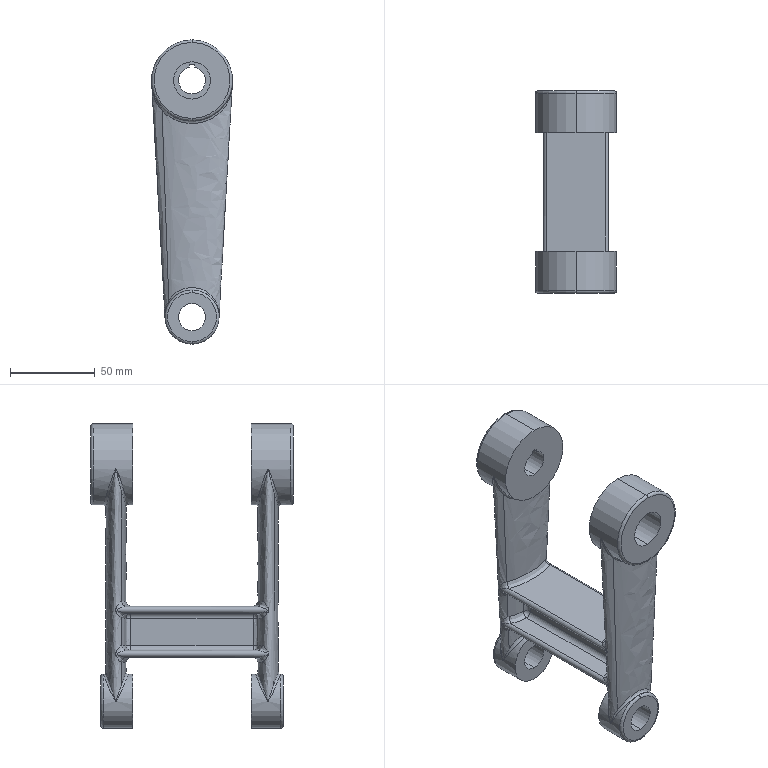Part | SolidWorks | features Boss 7, Cut 3, Fillet 3, Blend 2 | 1 solid | 113 faces | box 48 x 120 x 180 mm | volume 208513 mm3 | spline 46 | plane 27 | cylinder 24 | torus 8 | sphere 8 | commonest cylinder face diameters 16 x6 4 x4 6 x4 32 x4 48 x4 22 x2